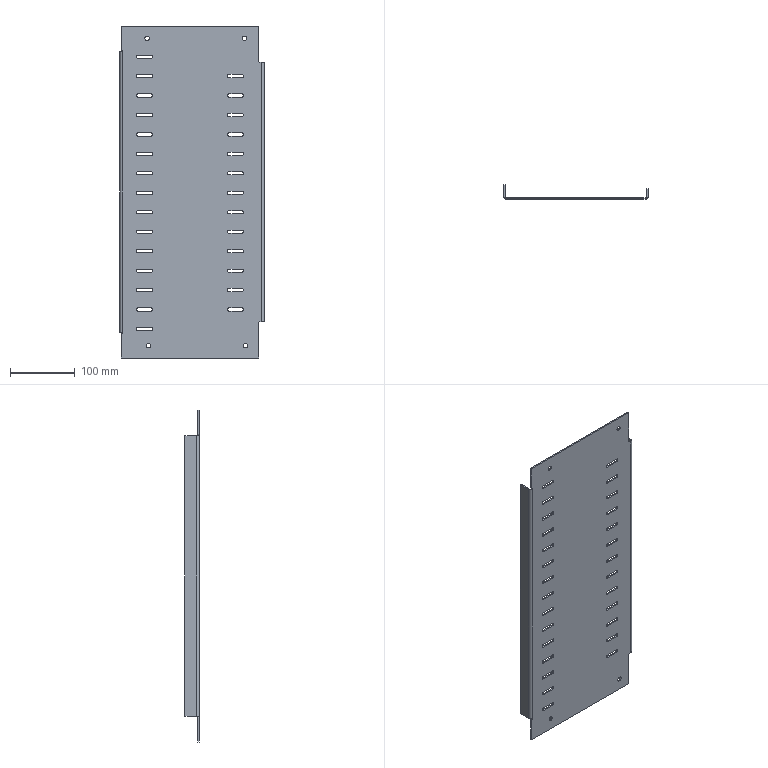Part | STEP file | 68336503 | 1 solid | 154 faces | box 222.5 x 22 x 512 mm | volume 244893 mm3 | plane 80 | cylinder 72 | spline 2 | commonest cylinder face diameters 5 x56 7 x10 3 x4 4 x2